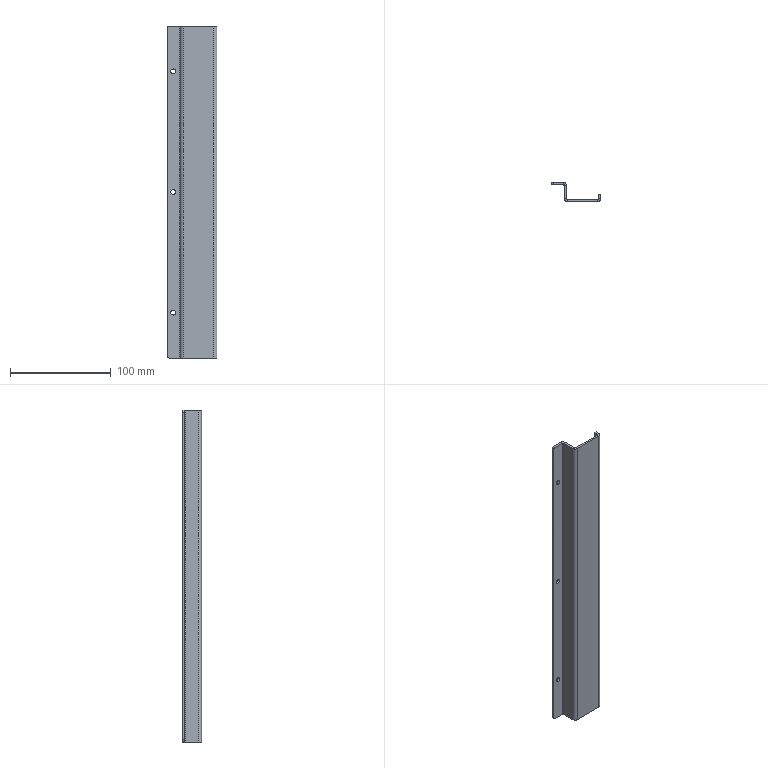Part | STEP file | 1 solid | 38 faces | box 49.5 x 19 x 330 mm | volume 45387 mm3 | plane 24 | cylinder 14 | commonest cylinder face diameters 4.6 x6 2 x3 6 x3 4 x2